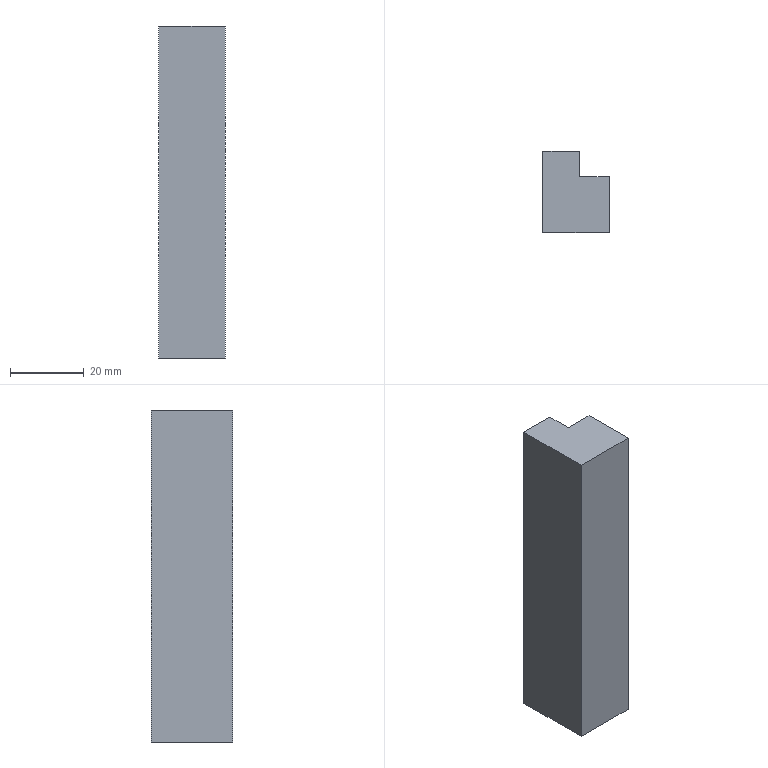Part | STEP file | 001-009-Riveting mechanism pressure plate | 1 solid | 8 faces | box 18 x 22 x 90 mm | volume 30600 mm3 | plane 8
STEP:
#1=CARTESIAN_POINT('',(0.,0.,0.));
#2=DIRECTION('',(0.,0.,1.));
#3=DIRECTION('',(1.,0.,0.));
#4=AXIS2_PLACEMENT_3D('',#1,#2,#3);
#5=CARTESIAN_POINT('',(9.,-11.,0.));
#6=VERTEX_POINT('',#5);
#7=CARTESIAN_POINT('',(9.,4.,0.));
#8=VERTEX_POINT('',#7);
#9=CARTESIAN_POINT('',(9.,-11.,0.));
#10=DIRECTION('',(0.,1.,0.));
#11=VECTOR('',#10,1.);
#12=LINE('',#9,#11);
#13=CARTESIAN_POINT('',(9.,-11.,90.));
#14=DIRECTION('',(-1.,0.,0.));
#15=DIRECTION('',(0.,-1.,0.));
#16=AXIS2_PLACEMENT_3D('',#13,#14,#15);
#17=PLANE('',#16);
#18=CARTESIAN_POINT('',(0.,-90.));
#19=DIRECTION('',(-1.,0.));
#20=VECTOR('',#19,1.);
#21=LINE('',#18,#20);
#22=(GEOMETRIC_REPRESENTATION_CONTEXT(2)PARAMETRIC_REPRESENTATION_CONTEXT()REPRESENTATION_CONTEXT('',''));
#23=DEFINITIONAL_REPRESENTATION('',(#21),#22);
#24=PCURVE('',#17,#23);
#25=CARTESIAN_POINT('',(0.,0.,0.));
#26=DIRECTION('',(0.,0.,-1.));
#27=DIRECTION('',(-1.,0.,0.));
#28=AXIS2_PLACEMENT_3D('',#25,#26,#27);
#29=PLANE('',#28);
#30=CARTESIAN_POINT('',(-9.,-11.));
#31=DIRECTION('',(0.,1.));
#32=VECTOR('',#31,1.);
#33=LINE('',#30,#32);
#34=(GEOMETRIC_REPRESENTATION_CONTEXT(2)PARAMETRIC_REPRESENTATION_CONTEXT()REPRESENTATION_CONTEXT('',''));
#35=DEFINITIONAL_REPRESENTATION('',(#33),#34);
#36=PCURVE('',#29,#35);
#37=SURFACE_CURVE('',#12,(#24,#36),.PCURVE_S1.);
#38=EDGE_CURVE('',#6,#8,#37,.T.);
#39=ORIENTED_EDGE('',*,*,#38,.T.);
#40=CARTESIAN_POINT('',(9.,4.,90.));
#41=VERTEX_POINT('',#40);
#42=CARTESIAN_POINT('',(9.,4.,0.));
#43=DIRECTION('',(0.,0.,1.));
#44=VECTOR('',#43,1.);
#45=LINE('',#42,#44);
#46=CARTESIAN_POINT('',(-15.,-90.));
#47=DIRECTION('',(0.,1.));
#48=VECTOR('',#47,1.);
#49=LINE('',#46,#48);
#50=(GEOMETRIC_REPRESENTATION_CONTEXT(2)PARAMETRIC_REPRESENTATION_CONTEXT()REPRESENTATION_CONTEXT('',''));
#51=DEFINITIONAL_REPRESENTATION('',(#49),#50);
#52=PCURVE('',#17,#51);
#53=CARTESIAN_POINT('',(9.,4.,0.));
#54=DIRECTION('',(0.,-1.,0.));
#55=DIRECTION('',(1.,0.,0.));
#56=AXIS2_PLACEMENT_3D('',#53,#54,#55);
#57=PLANE('',#56);
#58=CARTESIAN_POINT('',(0.,0.));
#59=DIRECTION('',(0.,1.));
#60=VECTOR('',#59,1.);
#61=LINE('',#58,#60);
#62=(GEOMETRIC_REPRESENTATION_CONTEXT(2)PARAMETRIC_REPRESENTATION_CONTEXT()REPRESENTATION_CONTEXT('',''));
#63=DEFINITIONAL_REPRESENTATION('',(#61),#62);
#64=PCURVE('',#57,#63);
#65=SURFACE_CURVE('',#45,(#52,#64),.PCURVE_S1.);
#66=EDGE_CURVE('',#8,#41,#65,.T.);
#67=ORIENTED_EDGE('',*,*,#66,.T.);
#68=CARTESIAN_POINT('',(9.,-11.,90.));
#69=VERTEX_POINT('',#68);
#70=CARTESIAN_POINT('',(9.,-11.,90.));
#71=DIRECTION('',(0.,1.,0.));
#72=VECTOR('',#71,1.);
#73=LINE('',#70,#72);
#74=CARTESIAN_POINT('',(0.,0.));
#75=DIRECTION('',(-1.,0.));
#76=VECTOR('',#75,1.);
#77=LINE('',#74,#76);
#78=(GEOMETRIC_REPRESENTATION_CONTEXT(2)PARAMETRIC_REPRESENTATION_CONTEXT()REPRESENTATION_CONTEXT('',''));
#79=DEFINITIONAL_REPRESENTATION('',(#77),#78);
#80=PCURVE('',#17,#79);
#81=CARTESIAN_POINT('',(0.,0.,90.));
#82=DIRECTION('',(0.,0.,-1.));
#83=DIRECTION('',(-1.,0.,0.));
#84=AXIS2_PLACEMENT_3D('',#81,#82,#83);
#85=PLANE('',#84);
#86=CARTESIAN_POINT('',(-9.,-11.));
#87=DIRECTION('',(0.,1.));
#88=VECTOR('',#87,1.);
#89=LINE('',#86,#88);
#90=(GEOMETRIC_REPRESENTATION_CONTEXT(2)PARAMETRIC_REPRESENTATION_CONTEXT()REPRESENTATION_CONTEXT('',''));
#91=DEFINITIONAL_REPRESENTATION('',(#89),#90);
#92=PCURVE('',#85,#91);
#93=SURFACE_CURVE('',#73,(#80,#92),.PCURVE_S1.);
#94=EDGE_CURVE('',#69,#41,#93,.T.);
#95=ORIENTED_EDGE('',*,*,#94,.F.);
#96=CARTESIAN_POINT('',(9.,-11.,90.));
#97=DIRECTION('',(0.,0.,-1.));
#98=VECTOR('',#97,1.);
#99=LINE('',#96,#98);
#100=CARTESIAN_POINT('',(0.,0.));
#101=DIRECTION('',(0.,-1.));
#102=VECTOR('',#101,1.);
#103=LINE('',#100,#102);
#104=(GEOMETRIC_REPRESENTATION_CONTEXT(2)PARAMETRIC_REPRESENTATION_CONTEXT()REPRESENTATION_CONTEXT('',''));
#105=DEFINITIONAL_REPRESENTATION('',(#103),#104);
#106=PCURVE('',#17,#105);
#107=CARTESIAN_POINT('',(-9.,-11.,90.));
#108=DIRECTION('',(0.,1.,0.));
#109=DIRECTION('',(0.,0.,1.));
#110=AXIS2_PLACEMENT_3D('',#107,#108,#109);
#111=PLANE('',#110);
#112=CARTESIAN_POINT('',(0.,18.));
#113=DIRECTION('',(-1.,0.));
#114=VECTOR('',#113,1.);
#115=LINE('',#112,#114);
#116=(GEOMETRIC_REPRESENTATION_CONTEXT(2)PARAMETRIC_REPRESENTATION_CONTEXT()REPRESENTATION_CONTEXT('',''));
#117=DEFINITIONAL_REPRESENTATION('',(#115),#116);
#118=PCURVE('',#111,#117);
#119=SURFACE_CURVE('',#99,(#106,#118),.PCURVE_S1.);
#120=EDGE_CURVE('',#69,#6,#119,.T.);
#121=ORIENTED_EDGE('',*,*,#120,.T.);
#122=EDGE_LOOP('',(#39,#67,#95,#121));
#123=FACE_BOUND('',#122,.T.);
#124=ADVANCED_FACE('',(#123),#17,.F.);
#125=CARTESIAN_POINT('',(1.,11.,90.));
#126=VERTEX_POINT('',#125);
#127=CARTESIAN_POINT('',(-9.,11.,90.));
#128=VERTEX_POINT('',#127);
#129=CARTESIAN_POINT('',(-9.,11.,90.));
#130=DIRECTION('',(-1.,0.,0.));
#131=VECTOR('',#130,1.);
#132=LINE('',#129,#131);
#133=CARTESIAN_POINT('',(-9.,11.,90.));
#134=DIRECTION('',(0.,-1.,0.));
#135=DIRECTION('',(1.,0.,0.));
#136=AXIS2_PLACEMENT_3D('',#133,#134,#135);
#137=PLANE('',#136);
#138=CARTESIAN_POINT('',(0.,0.));
#139=DIRECTION('',(-1.,0.));
#140=VECTOR('',#139,1.);
#141=LINE('',#138,#140);
#142=(GEOMETRIC_REPRESENTATION_CONTEXT(2)PARAMETRIC_REPRESENTATION_CONTEXT()REPRESENTATION_CONTEXT('',''));
#143=DEFINITIONAL_REPRESENTATION('',(#141),#142);
#144=PCURVE('',#137,#143);
#145=CARTESIAN_POINT('',(9.,11.));
#146=DIRECTION('',(1.,0.));
#147=VECTOR('',#146,1.);
#148=LINE('',#145,#147);
#149=(GEOMETRIC_REPRESENTATION_CONTEXT(2)PARAMETRIC_REPRESENTATION_CONTEXT()REPRESENTATION_CONTEXT('',''));
#150=DEFINITIONAL_REPRESENTATION('',(#148),#149);
#151=PCURVE('',#85,#150);
#152=SURFACE_CURVE('',#132,(#144,#151),.PCURVE_S1.);
#153=EDGE_CURVE('',#126,#128,#152,.T.);
#154=ORIENTED_EDGE('',*,*,#153,.F.);
#155=CARTESIAN_POINT('',(1.,11.,0.));
#156=VERTEX_POINT('',#155);
#157=CARTESIAN_POINT('',(1.,11.,0.));
#158=DIRECTION('',(0.,0.,1.));
#159=VECTOR('',#158,1.);
#160=LINE('',#157,#159);
#161=CARTESIAN_POINT('',(10.,-90.));
#162=DIRECTION('',(0.,1.));
#163=VECTOR('',#162,1.);
#164=LINE('',#161,#163);
#165=(GEOMETRIC_REPRESENTATION_CONTEXT(2)PARAMETRIC_REPRESENTATION_CONTEXT()REPRESENTATION_CONTEXT('',''));
#166=DEFINITIONAL_REPRESENTATION('',(#164),#165);
#167=PCURVE('',#137,#166);
#168=CARTESIAN_POINT('',(1.,11.,0.));
#169=DIRECTION('',(-1.,0.,0.));
#170=DIRECTION('',(0.,0.,1.));
#171=AXIS2_PLACEMENT_3D('',#168,#169,#170);
#172=PLANE('',#171);
#173=CARTESIAN_POINT('',(0.,0.));
#174=DIRECTION('',(1.,0.));
#175=VECTOR('',#174,1.);
#176=LINE('',#173,#175);
#177=(GEOMETRIC_REPRESENTATION_CONTEXT(2)PARAMETRIC_REPRESENTATION_CONTEXT()REPRESENTATION_CONTEXT('',''));
#178=DEFINITIONAL_REPRESENTATION('',(#176),#177);
#179=PCURVE('',#172,#178);
#180=SURFACE_CURVE('',#160,(#167,#179),.PCURVE_S1.);
#181=EDGE_CURVE('',#156,#126,#180,.T.);
#182=ORIENTED_EDGE('',*,*,#181,.F.);
#183=CARTESIAN_POINT('',(-9.,11.,0.));
#184=VERTEX_POINT('',#183);
#185=CARTESIAN_POINT('',(-9.,11.,0.));
#186=DIRECTION('',(-1.,0.,0.));
#187=VECTOR('',#186,1.);
#188=LINE('',#185,#187);
#189=CARTESIAN_POINT('',(0.,-90.));
#190=DIRECTION('',(-1.,0.));
#191=VECTOR('',#190,1.);
#192=LINE('',#189,#191);
#193=(GEOMETRIC_REPRESENTATION_CONTEXT(2)PARAMETRIC_REPRESENTATION_CONTEXT()REPRESENTATION_CONTEXT('',''));
#194=DEFINITIONAL_REPRESENTATION('',(#192),#193);
#195=PCURVE('',#137,#194);
#196=CARTESIAN_POINT('',(9.,11.));
#197=DIRECTION('',(1.,0.));
#198=VECTOR('',#197,1.);
#199=LINE('',#196,#198);
#200=(GEOMETRIC_REPRESENTATION_CONTEXT(2)PARAMETRIC_REPRESENTATION_CONTEXT()REPRESENTATION_CONTEXT('',''));
#201=DEFINITIONAL_REPRESENTATION('',(#199),#200);
#202=PCURVE('',#29,#201);
#203=SURFACE_CURVE('',#188,(#195,#202),.PCURVE_S1.);
#204=EDGE_CURVE('',#156,#184,#203,.T.);
#205=ORIENTED_EDGE('',*,*,#204,.T.);
#206=CARTESIAN_POINT('',(-9.,11.,90.));
#207=DIRECTION('',(0.,0.,-1.));
#208=VECTOR('',#207,1.);
#209=LINE('',#206,#208);
#210=CARTESIAN_POINT('',(0.,0.));
#211=DIRECTION('',(0.,-1.));
#212=VECTOR('',#211,1.);
#213=LINE('',#210,#212);
#214=(GEOMETRIC_REPRESENTATION_CONTEXT(2)PARAMETRIC_REPRESENTATION_CONTEXT()REPRESENTATION_CONTEXT('',''));
#215=DEFINITIONAL_REPRESENTATION('',(#213),#214);
#216=PCURVE('',#137,#215);
#217=CARTESIAN_POINT('',(-9.,-11.,90.));
#218=DIRECTION('',(1.,0.,0.));
#219=DIRECTION('',(0.,0.,-1.));
#220=AXIS2_PLACEMENT_3D('',#217,#218,#219);
#221=PLANE('',#220);
#222=CARTESIAN_POINT('',(0.,22.));
#223=DIRECTION('',(1.,0.));
#224=VECTOR('',#223,1.);
#225=LINE('',#222,#224);
#226=(GEOMETRIC_REPRESENTATION_CONTEXT(2)PARAMETRIC_REPRESENTATION_CONTEXT()REPRESENTATION_CONTEXT('',''));
#227=DEFINITIONAL_REPRESENTATION('',(#225),#226);
#228=PCURVE('',#221,#227);
#229=SURFACE_CURVE('',#209,(#216,#228),.PCURVE_S1.);
#230=EDGE_CURVE('',#128,#184,#229,.T.);
#231=ORIENTED_EDGE('',*,*,#230,.F.);
#232=EDGE_LOOP('',(#154,#182,#205,#231));
#233=FACE_BOUND('',#232,.T.);
#234=ADVANCED_FACE('',(#233),#137,.F.);
#235=CARTESIAN_POINT('',(-9.,-11.,0.));
#236=VERTEX_POINT('',#235);
#237=CARTESIAN_POINT('',(-9.,-11.,0.));
#238=DIRECTION('',(0.,-1.,0.));
#239=VECTOR('',#238,1.);
#240=LINE('',#237,#239);
#241=CARTESIAN_POINT('',(90.,0.));
#242=DIRECTION('',(0.,-1.));
#243=VECTOR('',#242,1.);
#244=LINE('',#241,#243);
#245=(GEOMETRIC_REPRESENTATION_CONTEXT(2)PARAMETRIC_REPRESENTATION_CONTEXT()REPRESENTATION_CONTEXT('',''));
#246=DEFINITIONAL_REPRESENTATION('',(#244),#245);
#247=PCURVE('',#221,#246);
#248=CARTESIAN_POINT('',(9.,-11.));
#249=DIRECTION('',(0.,-1.));
#250=VECTOR('',#249,1.);
#251=LINE('',#248,#250);
#252=(GEOMETRIC_REPRESENTATION_CONTEXT(2)PARAMETRIC_REPRESENTATION_CONTEXT()REPRESENTATION_CONTEXT('',''));
#253=DEFINITIONAL_REPRESENTATION('',(#251),#252);
#254=PCURVE('',#29,#253);
#255=SURFACE_CURVE('',#240,(#247,#254),.PCURVE_S1.);
#256=EDGE_CURVE('',#184,#236,#255,.T.);
#257=ORIENTED_EDGE('',*,*,#256,.T.);
#258=CARTESIAN_POINT('',(-9.,-11.,90.));
#259=VERTEX_POINT('',#258);
#260=CARTESIAN_POINT('',(-9.,-11.,90.));
#261=DIRECTION('',(0.,0.,-1.));
#262=VECTOR('',#261,1.);
#263=LINE('',#260,#262);
#264=CARTESIAN_POINT('',(0.,0.));
#265=DIRECTION('',(1.,0.));
#266=VECTOR('',#265,1.);
#267=LINE('',#264,#266);
#268=(GEOMETRIC_REPRESENTATION_CONTEXT(2)PARAMETRIC_REPRESENTATION_CONTEXT()REPRESENTATION_CONTEXT('',''));
#269=DEFINITIONAL_REPRESENTATION('',(#267),#268);
#270=PCURVE('',#221,#269);
#271=CARTESIAN_POINT('',(0.,0.));
#272=DIRECTION('',(-1.,0.));
#273=VECTOR('',#272,1.);
#274=LINE('',#271,#273);
#275=(GEOMETRIC_REPRESENTATION_CONTEXT(2)PARAMETRIC_REPRESENTATION_CONTEXT()REPRESENTATION_CONTEXT('',''));
#276=DEFINITIONAL_REPRESENTATION('',(#274),#275);
#277=PCURVE('',#111,#276);
#278=SURFACE_CURVE('',#263,(#270,#277),.PCURVE_S1.);
#279=EDGE_CURVE('',#259,#236,#278,.T.);
#280=ORIENTED_EDGE('',*,*,#279,.F.);
#281=CARTESIAN_POINT('',(-9.,-11.,90.));
#282=DIRECTION('',(0.,-1.,0.));
#283=VECTOR('',#282,1.);
#284=LINE('',#281,#283);
#285=CARTESIAN_POINT('',(0.,0.));
#286=DIRECTION('',(0.,-1.));
#287=VECTOR('',#286,1.);
#288=LINE('',#285,#287);
#289=(GEOMETRIC_REPRESENTATION_CONTEXT(2)PARAMETRIC_REPRESENTATION_CONTEXT()REPRESENTATION_CONTEXT('',''));
#290=DEFINITIONAL_REPRESENTATION('',(#288),#289);
#291=PCURVE('',#221,#290);
#292=CARTESIAN_POINT('',(9.,-11.));
#293=DIRECTION('',(0.,-1.));
#294=VECTOR('',#293,1.);
#295=LINE('',#292,#294);
#296=(GEOMETRIC_REPRESENTATION_CONTEXT(2)PARAMETRIC_REPRESENTATION_CONTEXT()REPRESENTATION_CONTEXT('',''));
#297=DEFINITIONAL_REPRESENTATION('',(#295),#296);
#298=PCURVE('',#85,#297);
#299=SURFACE_CURVE('',#284,(#291,#298),.PCURVE_S1.);
#300=EDGE_CURVE('',#128,#259,#299,.T.);
#301=ORIENTED_EDGE('',*,*,#300,.F.);
#302=ORIENTED_EDGE('',*,*,#230,.T.);
#303=EDGE_LOOP('',(#257,#280,#301,#302));
#304=FACE_BOUND('',#303,.T.);
#305=ADVANCED_FACE('',(#304),#221,.F.);
#306=CARTESIAN_POINT('',(-9.,-11.,0.));
#307=DIRECTION('',(1.,0.,0.));
#308=VECTOR('',#307,1.);
#309=LINE('',#306,#308);
#310=CARTESIAN_POINT('',(-90.,0.));
#311=DIRECTION('',(0.,1.));
#312=VECTOR('',#311,1.);
#313=LINE('',#310,#312);
#314=(GEOMETRIC_REPRESENTATION_CONTEXT(2)PARAMETRIC_REPRESENTATION_CONTEXT()REPRESENTATION_CONTEXT('',''));
#315=DEFINITIONAL_REPRESENTATION('',(#313),#314);
#316=PCURVE('',#111,#315);
#317=CARTESIAN_POINT('',(9.,-11.));
#318=DIRECTION('',(-1.,0.));
#319=VECTOR('',#318,1.);
#320=LINE('',#317,#319);
#321=(GEOMETRIC_REPRESENTATION_CONTEXT(2)PARAMETRIC_REPRESENTATION_CONTEXT()REPRESENTATION_CONTEXT('',''));
#322=DEFINITIONAL_REPRESENTATION('',(#320),#321);
#323=PCURVE('',#29,#322);
#324=SURFACE_CURVE('',#309,(#316,#323),.PCURVE_S1.);
#325=EDGE_CURVE('',#236,#6,#324,.T.);
#326=ORIENTED_EDGE('',*,*,#325,.T.);
#327=ORIENTED_EDGE('',*,*,#120,.F.);
#328=CARTESIAN_POINT('',(-9.,-11.,90.));
#329=DIRECTION('',(1.,0.,0.));
#330=VECTOR('',#329,1.);
#331=LINE('',#328,#330);
#332=CARTESIAN_POINT('',(0.,0.));
#333=DIRECTION('',(0.,1.));
#334=VECTOR('',#333,1.);
#335=LINE('',#332,#334);
#336=(GEOMETRIC_REPRESENTATION_CONTEXT(2)PARAMETRIC_REPRESENTATION_CONTEXT()REPRESENTATION_CONTEXT('',''));
#337=DEFINITIONAL_REPRESENTATION('',(#335),#336);
#338=PCURVE('',#111,#337);
#339=CARTESIAN_POINT('',(9.,-11.));
#340=DIRECTION('',(-1.,0.));
#341=VECTOR('',#340,1.);
#342=LINE('',#339,#341);
#343=(GEOMETRIC_REPRESENTATION_CONTEXT(2)PARAMETRIC_REPRESENTATION_CONTEXT()REPRESENTATION_CONTEXT('',''));
#344=DEFINITIONAL_REPRESENTATION('',(#342),#343);
#345=PCURVE('',#85,#344);
#346=SURFACE_CURVE('',#331,(#338,#345),.PCURVE_S1.);
#347=EDGE_CURVE('',#259,#69,#346,.T.);
#348=ORIENTED_EDGE('',*,*,#347,.F.);
#349=ORIENTED_EDGE('',*,*,#279,.T.);
#350=EDGE_LOOP('',(#326,#327,#348,#349));
#351=FACE_BOUND('',#350,.T.);
#352=ADVANCED_FACE('',(#351),#111,.F.);
#353=ORIENTED_EDGE('',*,*,#94,.T.);
#354=CARTESIAN_POINT('',(1.,4.,90.));
#355=VERTEX_POINT('',#354);
#356=CARTESIAN_POINT('',(9.,4.,90.));
#357=DIRECTION('',(1.,0.,0.));
#358=VECTOR('',#357,1.);
#359=LINE('',#356,#358);
#360=CARTESIAN_POINT('',(-9.,4.));
#361=DIRECTION('',(-1.,0.));
#362=VECTOR('',#361,1.);
#363=LINE('',#360,#362);
#364=(GEOMETRIC_REPRESENTATION_CONTEXT(2)PARAMETRIC_REPRESENTATION_CONTEXT()REPRESENTATION_CONTEXT('',''));
#365=DEFINITIONAL_REPRESENTATION('',(#363),#364);
#366=PCURVE('',#85,#365);
#367=CARTESIAN_POINT('',(0.,90.));
#368=DIRECTION('',(1.,0.));
#369=VECTOR('',#368,1.);
#370=LINE('',#367,#369);
#371=(GEOMETRIC_REPRESENTATION_CONTEXT(2)PARAMETRIC_REPRESENTATION_CONTEXT()REPRESENTATION_CONTEXT('',''));
#372=DEFINITIONAL_REPRESENTATION('',(#370),#371);
#373=PCURVE('',#57,#372);
#374=SURFACE_CURVE('',#359,(#366,#373),.PCURVE_S1.);
#375=EDGE_CURVE('',#355,#41,#374,.T.);
#376=ORIENTED_EDGE('',*,*,#375,.F.);
#377=CARTESIAN_POINT('',(1.,11.,90.));
#378=DIRECTION('',(0.,-1.,0.));
#379=VECTOR('',#378,1.);
#380=LINE('',#377,#379);
#381=CARTESIAN_POINT('',(-1.,11.));
#382=DIRECTION('',(0.,-1.));
#383=VECTOR('',#382,1.);
#384=LINE('',#381,#383);
#385=(GEOMETRIC_REPRESENTATION_CONTEXT(2)PARAMETRIC_REPRESENTATION_CONTEXT()REPRESENTATION_CONTEXT('',''));
#386=DEFINITIONAL_REPRESENTATION('',(#384),#385);
#387=PCURVE('',#85,#386);
#388=CARTESIAN_POINT('',(90.,0.));
#389=DIRECTION('',(0.,-1.));
#390=VECTOR('',#389,1.);
#391=LINE('',#388,#390);
#392=(GEOMETRIC_REPRESENTATION_CONTEXT(2)PARAMETRIC_REPRESENTATION_CONTEXT()REPRESENTATION_CONTEXT('',''));
#393=DEFINITIONAL_REPRESENTATION('',(#391),#392);
#394=PCURVE('',#172,#393);
#395=SURFACE_CURVE('',#380,(#387,#394),.PCURVE_S1.);
#396=EDGE_CURVE('',#126,#355,#395,.T.);
#397=ORIENTED_EDGE('',*,*,#396,.F.);
#398=ORIENTED_EDGE('',*,*,#153,.T.);
#399=ORIENTED_EDGE('',*,*,#300,.T.);
#400=ORIENTED_EDGE('',*,*,#347,.T.);
#401=EDGE_LOOP('',(#353,#376,#397,#398,#399,#400));
#402=FACE_BOUND('',#401,.T.);
#403=ADVANCED_FACE('',(#402),#85,.F.);
#404=CARTESIAN_POINT('',(1.,4.,0.));
#405=VERTEX_POINT('',#404);
#406=CARTESIAN_POINT('',(9.,4.,0.));
#407=DIRECTION('',(1.,0.,0.));
#408=VECTOR('',#407,1.);
#409=LINE('',#406,#408);
#410=CARTESIAN_POINT('',(-9.,4.));
#411=DIRECTION('',(-1.,0.));
#412=VECTOR('',#411,1.);
#413=LINE('',#410,#412);
#414=(GEOMETRIC_REPRESENTATION_CONTEXT(2)PARAMETRIC_REPRESENTATION_CONTEXT()REPRESENTATION_CONTEXT('',''));
#415=DEFINITIONAL_REPRESENTATION('',(#413),#414);
#416=PCURVE('',#29,#415);
#417=CARTESIAN_POINT('',(0.,0.));
#418=DIRECTION('',(1.,0.));
#419=VECTOR('',#418,1.);
#420=LINE('',#417,#419);
#421=(GEOMETRIC_REPRESENTATION_CONTEXT(2)PARAMETRIC_REPRESENTATION_CONTEXT()REPRESENTATION_CONTEXT('',''));
#422=DEFINITIONAL_REPRESENTATION('',(#420),#421);
#423=PCURVE('',#57,#422);
#424=SURFACE_CURVE('',#409,(#416,#423),.PCURVE_S1.);
#425=EDGE_CURVE('',#405,#8,#424,.T.);
#426=ORIENTED_EDGE('',*,*,#425,.T.);
#427=ORIENTED_EDGE('',*,*,#38,.F.);
#428=ORIENTED_EDGE('',*,*,#325,.F.);
#429=ORIENTED_EDGE('',*,*,#256,.F.);
#430=ORIENTED_EDGE('',*,*,#204,.F.);
#431=CARTESIAN_POINT('',(1.,11.,0.));
#432=DIRECTION('',(0.,-1.,0.));
#433=VECTOR('',#432,1.);
#434=LINE('',#431,#433);
#435=CARTESIAN_POINT('',(-1.,11.));
#436=DIRECTION('',(0.,-1.));
#437=VECTOR('',#436,1.);
#438=LINE('',#435,#437);
#439=(GEOMETRIC_REPRESENTATION_CONTEXT(2)PARAMETRIC_REPRESENTATION_CONTEXT()REPRESENTATION_CONTEXT('',''));
#440=DEFINITIONAL_REPRESENTATION('',(#438),#439);
#441=PCURVE('',#29,#440);
#442=CARTESIAN_POINT('',(0.,0.));
#443=DIRECTION('',(0.,-1.));
#444=VECTOR('',#443,1.);
#445=LINE('',#442,#444);
#446=(GEOMETRIC_REPRESENTATION_CONTEXT(2)PARAMETRIC_REPRESENTATION_CONTEXT()REPRESENTATION_CONTEXT('',''));
#447=DEFINITIONAL_REPRESENTATION('',(#445),#446);
#448=PCURVE('',#172,#447);
#449=SURFACE_CURVE('',#434,(#441,#448),.PCURVE_S1.);
#450=EDGE_CURVE('',#156,#405,#449,.T.);
#451=ORIENTED_EDGE('',*,*,#450,.T.);
#452=EDGE_LOOP('',(#426,#427,#428,#429,#430,#451));
#453=FACE_BOUND('',#452,.T.);
#454=ADVANCED_FACE('',(#453),#29,.T.);
#455=ORIENTED_EDGE('',*,*,#375,.T.);
#456=ORIENTED_EDGE('',*,*,#66,.F.);
#457=ORIENTED_EDGE('',*,*,#425,.F.);
#458=CARTESIAN_POINT('',(1.,4.,0.));
#459=DIRECTION('',(0.,0.,1.));
#460=VECTOR('',#459,1.);
#461=LINE('',#458,#460);
#462=CARTESIAN_POINT('',(-8.,0.));
#463=DIRECTION('',(0.,1.));
#464=VECTOR('',#463,1.);
#465=LINE('',#462,#464);
#466=(GEOMETRIC_REPRESENTATION_CONTEXT(2)PARAMETRIC_REPRESENTATION_CONTEXT()REPRESENTATION_CONTEXT('',''));
#467=DEFINITIONAL_REPRESENTATION('',(#465),#466);
#468=PCURVE('',#57,#467);
#469=CARTESIAN_POINT('',(0.,-7.));
#470=DIRECTION('',(1.,0.));
#471=VECTOR('',#470,1.);
#472=LINE('',#469,#471);
#473=(GEOMETRIC_REPRESENTATION_CONTEXT(2)PARAMETRIC_REPRESENTATION_CONTEXT()REPRESENTATION_CONTEXT('',''));
#474=DEFINITIONAL_REPRESENTATION('',(#472),#473);
#475=PCURVE('',#172,#474);
#476=SURFACE_CURVE('',#461,(#468,#475),.PCURVE_S1.);
#477=EDGE_CURVE('',#405,#355,#476,.T.);
#478=ORIENTED_EDGE('',*,*,#477,.T.);
#479=EDGE_LOOP('',(#455,#456,#457,#478));
#480=FACE_BOUND('',#479,.T.);
#481=ADVANCED_FACE('',(#480),#57,.F.);
#482=ORIENTED_EDGE('',*,*,#396,.T.);
#483=ORIENTED_EDGE('',*,*,#477,.F.);
#484=ORIENTED_EDGE('',*,*,#450,.F.);
#485=ORIENTED_EDGE('',*,*,#181,.T.);
#486=EDGE_LOOP('',(#482,#483,#484,#485));
#487=FACE_BOUND('',#486,.T.);
#488=ADVANCED_FACE('',(#487),#172,.F.);
#489=CLOSED_SHELL('',(#124,#234,#305,#352,#403,#454,#481,#488));
#490=MANIFOLD_SOLID_BREP('',#489);
#491=(LENGTH_UNIT()NAMED_UNIT(*)SI_UNIT(.MILLI.,.METRE.));
#492=UNCERTAINTY_MEASURE_WITH_UNIT(LENGTH_MEASURE(0.0000001),#491,'','');
#493=(NAMED_UNIT(*)PLANE_ANGLE_UNIT()SI_UNIT($,.RADIAN.));
#494=(NAMED_UNIT(*)SI_UNIT($,.STERADIAN.)SOLID_ANGLE_UNIT());
#495=(GEOMETRIC_REPRESENTATION_CONTEXT(3)GLOBAL_UNCERTAINTY_ASSIGNED_CONTEXT((#492))GLOBAL_UNIT_ASSIGNED_CONTEXT((#491,#493,#494))REPRESENTATION_CONTEXT('',''));
#496=ADVANCED_BREP_SHAPE_REPRESENTATION('',(#4,#490),#495);